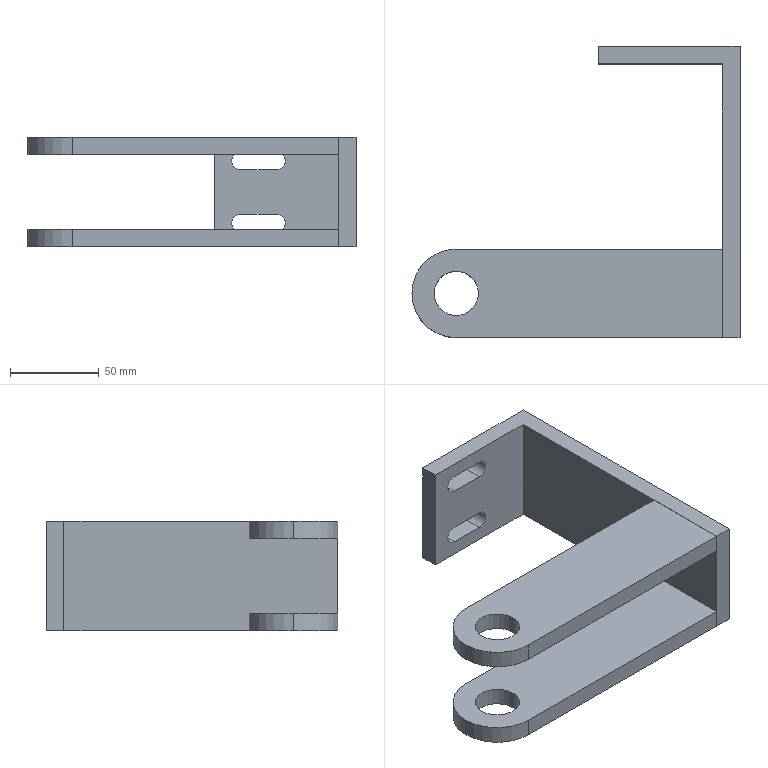Part | SolidWorks | features ICE 3, Extrusion 1, MirrorSolid 1, Split 1 | 3 solids | 34 faces | box 185 x 164.4 x 62 mm | volume 299575 mm3 | plane 22 | cylinder 12 | commonest cylinder face diameters 10 x4 25 x4 50 x4
STEP:
#1=CARTESIAN_POINT('',(-75.,25.,52.));
#2=VERTEX_POINT('',#1);
#3=CARTESIAN_POINT('',(-100.,0.,52.));
#4=VERTEX_POINT('',#3);
#5=CARTESIAN_POINT('',(-75.,0.,52.));
#6=DIRECTION('',(0.,0.,1.));
#7=DIRECTION('',(1.,0.,0.));
#8=AXIS2_PLACEMENT_3D('',#5,#6,#7);
#9=CIRCLE('',#8,25.);
#10=EDGE_CURVE('',#2,#4,#9,.T.);
#11=ORIENTED_EDGE('',*,*,#10,.T.);
#12=CARTESIAN_POINT('',(-100.,0.,62.));
#13=VERTEX_POINT('',#12);
#14=CARTESIAN_POINT('',(-100.,0.,52.));
#15=DIRECTION('',(0.,0.,1.));
#16=VECTOR('',#15,1000.);
#17=LINE('',#14,#16);
#18=EDGE_CURVE('',#4,#13,#17,.T.);
#19=ORIENTED_EDGE('',*,*,#18,.T.);
#20=CARTESIAN_POINT('',(-75.,25.,62.));
#21=VERTEX_POINT('',#20);
#22=CARTESIAN_POINT('',(-75.,0.,62.));
#23=DIRECTION('',(0.,0.,1.));
#24=DIRECTION('',(1.,0.,0.));
#25=AXIS2_PLACEMENT_3D('',#22,#23,#24);
#26=CIRCLE('',#25,25.);
#27=EDGE_CURVE('',#21,#13,#26,.T.);
#28=ORIENTED_EDGE('',*,*,#27,.F.);
#29=CARTESIAN_POINT('',(-75.,25.,52.));
#30=DIRECTION('',(0.,0.,1.));
#31=VECTOR('',#30,1000.);
#32=LINE('',#29,#31);
#33=EDGE_CURVE('',#2,#21,#32,.T.);
#34=ORIENTED_EDGE('',*,*,#33,.F.);
#35=EDGE_LOOP('',(#11,#19,#28,#34));
#36=FACE_OUTER_BOUND('',#35,.T.);
#37=CARTESIAN_POINT('',(-75.,0.,52.));
#38=DIRECTION('',(0.,0.,1.));
#39=DIRECTION('',(-1.,0.,0.));
#40=AXIS2_PLACEMENT_3D('',#37,#38,#39);
#41=CYLINDRICAL_SURFACE('',#40,25.);
#42=ADVANCED_FACE('',(#36),#41,.T.);
#43=CARTESIAN_POINT('',(-62.5,0.,52.));
#44=VERTEX_POINT('',#43);
#45=CARTESIAN_POINT('',(-87.5,0.,52.));
#46=VERTEX_POINT('',#45);
#47=CARTESIAN_POINT('',(-75.,0.,52.));
#48=DIRECTION('',(0.,0.,1.));
#49=DIRECTION('',(1.,0.,0.));
#50=AXIS2_PLACEMENT_3D('',#47,#48,#49);
#51=CIRCLE('',#50,12.5);
#52=EDGE_CURVE('',#44,#46,#51,.T.);
#53=ORIENTED_EDGE('',*,*,#52,.F.);
#54=CARTESIAN_POINT('',(-62.5,0.,62.));
#55=VERTEX_POINT('',#54);
#56=CARTESIAN_POINT('',(-62.5,0.,52.));
#57=DIRECTION('',(0.,0.,1.));
#58=VECTOR('',#57,1000.);
#59=LINE('',#56,#58);
#60=EDGE_CURVE('',#44,#55,#59,.T.);
#61=ORIENTED_EDGE('',*,*,#60,.T.);
#62=CARTESIAN_POINT('',(-87.5,0.,62.));
#63=VERTEX_POINT('',#62);
#64=CARTESIAN_POINT('',(-75.,0.,62.));
#65=DIRECTION('',(0.,0.,1.));
#66=DIRECTION('',(1.,0.,0.));
#67=AXIS2_PLACEMENT_3D('',#64,#65,#66);
#68=CIRCLE('',#67,12.5);
#69=EDGE_CURVE('',#55,#63,#68,.T.);
#70=ORIENTED_EDGE('',*,*,#69,.T.);
#71=CARTESIAN_POINT('',(-87.5,0.,52.));
#72=DIRECTION('',(0.,0.,1.));
#73=VECTOR('',#72,1000.);
#74=LINE('',#71,#73);
#75=EDGE_CURVE('',#46,#63,#74,.T.);
#76=ORIENTED_EDGE('',*,*,#75,.F.);
#77=EDGE_LOOP('',(#53,#61,#70,#76));
#78=FACE_OUTER_BOUND('',#77,.T.);
#79=CARTESIAN_POINT('',(-75.,0.,52.));
#80=DIRECTION('',(0.,0.,1.));
#81=DIRECTION('',(-1.,0.,0.));
#82=AXIS2_PLACEMENT_3D('',#79,#80,#81);
#83=CYLINDRICAL_SURFACE('',#82,12.5);
#84=ADVANCED_FACE('',(#78),#83,.F.);
#85=CARTESIAN_POINT('',(75.,-25.,52.));
#86=VERTEX_POINT('',#85);
#87=CARTESIAN_POINT('',(75.,-25.,62.));
#88=VERTEX_POINT('',#87);
#89=CARTESIAN_POINT('',(75.,-25.,10.));
#90=DIRECTION('',(0.,0.,1.));
#91=VECTOR('',#90,1000.);
#92=LINE('',#89,#91);
#93=EDGE_CURVE('',#86,#88,#92,.T.);
#94=ORIENTED_EDGE('',*,*,#93,.F.);
#95=CARTESIAN_POINT('',(75.,25.,52.));
#96=VERTEX_POINT('',#95);
#97=CARTESIAN_POINT('',(75.,0.,52.));
#98=DIRECTION('',(0.,-1.,0.));
#99=VECTOR('',#98,1000.);
#100=LINE('',#97,#99);
#101=EDGE_CURVE('',#96,#86,#100,.T.);
#102=ORIENTED_EDGE('',*,*,#101,.F.);
#103=CARTESIAN_POINT('',(75.,25.,62.));
#104=VERTEX_POINT('',#103);
#105=CARTESIAN_POINT('',(75.,25.,52.));
#106=DIRECTION('',(0.,0.,1.));
#107=VECTOR('',#106,1000.);
#108=LINE('',#105,#107);
#109=EDGE_CURVE('',#96,#104,#108,.T.);
#110=ORIENTED_EDGE('',*,*,#109,.T.);
#111=CARTESIAN_POINT('',(75.,-25.,62.));
#112=DIRECTION('',(0.,1.,0.));
#113=VECTOR('',#112,1000.);
#114=LINE('',#111,#113);
#115=EDGE_CURVE('',#88,#104,#114,.T.);
#116=ORIENTED_EDGE('',*,*,#115,.F.);
#117=EDGE_LOOP('',(#94,#102,#110,#116));
#118=FACE_OUTER_BOUND('',#117,.T.);
#119=CARTESIAN_POINT('',(75.,129.4,0.));
#120=DIRECTION('',(-1.,0.,0.));
#121=DIRECTION('',(0.,0.,1.));
#122=AXIS2_PLACEMENT_3D('',#119,#120,#121);
#123=PLANE('',#122);
#124=ADVANCED_FACE('',(#118),#123,.F.);
#125=CARTESIAN_POINT('',(-75.,-25.,52.));
#126=VERTEX_POINT('',#125);
#127=CARTESIAN_POINT('',(0.,-25.,52.));
#128=DIRECTION('',(1.,0.,0.));
#129=VECTOR('',#128,1000.);
#130=LINE('',#127,#129);
#131=EDGE_CURVE('',#126,#86,#130,.T.);
#132=ORIENTED_EDGE('',*,*,#131,.F.);
#133=CARTESIAN_POINT('',(-75.,0.,52.));
#134=DIRECTION('',(0.,0.,1.));
#135=DIRECTION('',(1.,0.,0.));
#136=AXIS2_PLACEMENT_3D('',#133,#134,#135);
#137=CIRCLE('',#136,25.);
#138=EDGE_CURVE('',#4,#126,#137,.T.);
#139=ORIENTED_EDGE('',*,*,#138,.F.);
#140=ORIENTED_EDGE('',*,*,#10,.F.);
#141=CARTESIAN_POINT('',(0.,25.,52.));
#142=DIRECTION('',(1.,0.,0.));
#143=VECTOR('',#142,1000.);
#144=LINE('',#141,#143);
#145=EDGE_CURVE('',#2,#96,#144,.T.);
#146=ORIENTED_EDGE('',*,*,#145,.T.);
#147=ORIENTED_EDGE('',*,*,#101,.T.);
#148=EDGE_LOOP('',(#132,#139,#140,#146,#147));
#149=FACE_OUTER_BOUND('',#148,.T.);
#150=CARTESIAN_POINT('',(-75.,0.,52.));
#151=DIRECTION('',(0.,0.,1.));
#152=DIRECTION('',(1.,0.,0.));
#153=AXIS2_PLACEMENT_3D('',#150,#151,#152);
#154=CIRCLE('',#153,12.5);
#155=EDGE_CURVE('',#46,#44,#154,.T.);
#156=ORIENTED_EDGE('',*,*,#155,.T.);
#157=ORIENTED_EDGE('',*,*,#52,.T.);
#158=EDGE_LOOP('',(#156,#157));
#159=FACE_BOUND('',#158,.T.);
#160=CARTESIAN_POINT('',(0.,0.,52.));
#161=DIRECTION('',(0.,0.,-1.));
#162=DIRECTION('',(1.,0.,0.));
#163=AXIS2_PLACEMENT_3D('',#160,#161,#162);
#164=PLANE('',#163);
#165=ADVANCED_FACE('',(#149,#159),#164,.T.);
#166=ORIENTED_EDGE('',*,*,#131,.T.);
#167=ORIENTED_EDGE('',*,*,#93,.T.);
#168=CARTESIAN_POINT('',(-75.,-25.,62.));
#169=VERTEX_POINT('',#168);
#170=CARTESIAN_POINT('',(85.,-25.,62.));
#171=DIRECTION('',(-1.,0.,0.));
#172=VECTOR('',#171,1000.);
#173=LINE('',#170,#172);
#174=EDGE_CURVE('',#88,#169,#173,.T.);
#175=ORIENTED_EDGE('',*,*,#174,.T.);
#176=CARTESIAN_POINT('',(-75.,-25.,52.));
#177=DIRECTION('',(0.,0.,1.));
#178=VECTOR('',#177,1000.);
#179=LINE('',#176,#178);
#180=EDGE_CURVE('',#126,#169,#179,.T.);
#181=ORIENTED_EDGE('',*,*,#180,.F.);
#182=EDGE_LOOP('',(#166,#167,#175,#181));
#183=FACE_OUTER_BOUND('',#182,.T.);
#184=CARTESIAN_POINT('',(0.,-25.,10.));
#185=DIRECTION('',(0.,1.,0.));
#186=DIRECTION('',(-1.,0.,0.));
#187=AXIS2_PLACEMENT_3D('',#184,#185,#186);
#188=PLANE('',#187);
#189=ADVANCED_FACE('',(#183),#188,.F.);
#190=ORIENTED_EDGE('',*,*,#18,.F.);
#191=ORIENTED_EDGE('',*,*,#138,.T.);
#192=ORIENTED_EDGE('',*,*,#180,.T.);
#193=CARTESIAN_POINT('',(-75.,0.,62.));
#194=DIRECTION('',(0.,0.,1.));
#195=DIRECTION('',(1.,0.,0.));
#196=AXIS2_PLACEMENT_3D('',#193,#194,#195);
#197=CIRCLE('',#196,25.);
#198=EDGE_CURVE('',#13,#169,#197,.T.);
#199=ORIENTED_EDGE('',*,*,#198,.F.);
#200=EDGE_LOOP('',(#190,#191,#192,#199));
#201=FACE_OUTER_BOUND('',#200,.T.);
#202=CARTESIAN_POINT('',(-75.,0.,52.));
#203=DIRECTION('',(0.,0.,1.));
#204=DIRECTION('',(-1.,0.,0.));
#205=AXIS2_PLACEMENT_3D('',#202,#203,#204);
#206=CYLINDRICAL_SURFACE('',#205,25.);
#207=ADVANCED_FACE('',(#201),#206,.T.);
#208=CARTESIAN_POINT('',(0.,25.,62.));
#209=DIRECTION('',(1.,0.,0.));
#210=VECTOR('',#209,1000.);
#211=LINE('',#208,#210);
#212=EDGE_CURVE('',#21,#104,#211,.T.);
#213=ORIENTED_EDGE('',*,*,#212,.T.);
#214=ORIENTED_EDGE('',*,*,#109,.F.);
#215=ORIENTED_EDGE('',*,*,#145,.F.);
#216=ORIENTED_EDGE('',*,*,#33,.T.);
#217=EDGE_LOOP('',(#213,#214,#215,#216));
#218=FACE_OUTER_BOUND('',#217,.T.);
#219=CARTESIAN_POINT('',(0.,25.,52.));
#220=DIRECTION('',(0.,1.,0.));
#221=DIRECTION('',(-1.,0.,0.));
#222=AXIS2_PLACEMENT_3D('',#219,#220,#221);
#223=PLANE('',#222);
#224=ADVANCED_FACE('',(#218),#223,.T.);
#225=ORIENTED_EDGE('',*,*,#60,.F.);
#226=ORIENTED_EDGE('',*,*,#155,.F.);
#227=ORIENTED_EDGE('',*,*,#75,.T.);
#228=CARTESIAN_POINT('',(-75.,0.,62.));
#229=DIRECTION('',(0.,0.,1.));
#230=DIRECTION('',(1.,0.,0.));
#231=AXIS2_PLACEMENT_3D('',#228,#229,#230);
#232=CIRCLE('',#231,12.5);
#233=EDGE_CURVE('',#63,#55,#232,.T.);
#234=ORIENTED_EDGE('',*,*,#233,.T.);
#235=EDGE_LOOP('',(#225,#226,#227,#234));
#236=FACE_OUTER_BOUND('',#235,.T.);
#237=CARTESIAN_POINT('',(-75.,0.,52.));
#238=DIRECTION('',(0.,0.,1.));
#239=DIRECTION('',(-1.,0.,0.));
#240=AXIS2_PLACEMENT_3D('',#237,#238,#239);
#241=CYLINDRICAL_SURFACE('',#240,12.5);
#242=ADVANCED_FACE('',(#236),#241,.F.);
#243=ORIENTED_EDGE('',*,*,#233,.F.);
#244=ORIENTED_EDGE('',*,*,#69,.F.);
#245=EDGE_LOOP('',(#243,#244));
#246=FACE_BOUND('',#245,.T.);
#247=ORIENTED_EDGE('',*,*,#174,.F.);
#248=ORIENTED_EDGE('',*,*,#115,.T.);
#249=ORIENTED_EDGE('',*,*,#212,.F.);
#250=ORIENTED_EDGE('',*,*,#27,.T.);
#251=ORIENTED_EDGE('',*,*,#198,.T.);
#252=EDGE_LOOP('',(#247,#248,#249,#250,#251));
#253=FACE_OUTER_BOUND('',#252,.T.);
#254=CARTESIAN_POINT('',(85.,-25.,62.));
#255=DIRECTION('',(0.,0.,-1.));
#256=DIRECTION('',(-1.,0.,0.));
#257=AXIS2_PLACEMENT_3D('',#254,#255,#256);
#258=PLANE('',#257);
#259=ADVANCED_FACE('',(#246,#253),#258,.F.);
#260=CLOSED_SHELL('',(#42,#84,#124,#165,#189,#207,#224,#242,#259));
#261=MANIFOLD_SOLID_BREP('',#260);
#262=CARTESIAN_POINT('',(-87.5,0.,10.));
#263=VERTEX_POINT('',#262);
#264=CARTESIAN_POINT('',(-62.5,0.,10.));
#265=VERTEX_POINT('',#264);
#266=CARTESIAN_POINT('',(-75.,0.,10.));
#267=DIRECTION('',(0.,0.,1.));
#268=DIRECTION('',(1.,0.,0.));
#269=AXIS2_PLACEMENT_3D('',#266,#267,#268);
#270=CIRCLE('',#269,12.5);
#271=EDGE_CURVE('',#263,#265,#270,.T.);
#272=ORIENTED_EDGE('',*,*,#271,.T.);
#273=CARTESIAN_POINT('',(-62.5,0.,0.));
#274=VERTEX_POINT('',#273);
#275=CARTESIAN_POINT('',(-62.5,0.,10.));
#276=DIRECTION('',(0.,0.,-1.));
#277=VECTOR('',#276,1000.);
#278=LINE('',#275,#277);
#279=EDGE_CURVE('',#265,#274,#278,.T.);
#280=ORIENTED_EDGE('',*,*,#279,.T.);
#281=CARTESIAN_POINT('',(-87.5,0.,0.));
#282=VERTEX_POINT('',#281);
#283=CARTESIAN_POINT('',(-75.,0.,0.));
#284=DIRECTION('',(0.,0.,1.));
#285=DIRECTION('',(1.,0.,0.));
#286=AXIS2_PLACEMENT_3D('',#283,#284,#285);
#287=CIRCLE('',#286,12.5);
#288=EDGE_CURVE('',#282,#274,#287,.T.);
#289=ORIENTED_EDGE('',*,*,#288,.F.);
#290=CARTESIAN_POINT('',(-87.5,0.,10.));
#291=DIRECTION('',(0.,0.,-1.));
#292=VECTOR('',#291,1000.);
#293=LINE('',#290,#292);
#294=EDGE_CURVE('',#263,#282,#293,.T.);
#295=ORIENTED_EDGE('',*,*,#294,.F.);
#296=EDGE_LOOP('',(#272,#280,#289,#295));
#297=FACE_OUTER_BOUND('',#296,.T.);
#298=CARTESIAN_POINT('',(-75.,0.,10.));
#299=DIRECTION('',(0.,0.,-1.));
#300=DIRECTION('',(-1.,0.,0.));
#301=AXIS2_PLACEMENT_3D('',#298,#299,#300);
#302=CYLINDRICAL_SURFACE('',#301,12.5);
#303=ADVANCED_FACE('',(#297),#302,.F.);
#304=CARTESIAN_POINT('',(-100.,0.,10.));
#305=VERTEX_POINT('',#304);
#306=CARTESIAN_POINT('',(-75.,-25.,10.));
#307=VERTEX_POINT('',#306);
#308=CARTESIAN_POINT('',(-75.,0.,10.));
#309=DIRECTION('',(0.,0.,1.));
#310=DIRECTION('',(1.,0.,0.));
#311=AXIS2_PLACEMENT_3D('',#308,#309,#310);
#312=CIRCLE('',#311,25.);
#313=EDGE_CURVE('',#305,#307,#312,.T.);
#314=ORIENTED_EDGE('',*,*,#313,.F.);
#315=CARTESIAN_POINT('',(-100.,0.,0.));
#316=VERTEX_POINT('',#315);
#317=CARTESIAN_POINT('',(-100.,0.,10.));
#318=DIRECTION('',(0.,0.,-1.));
#319=VECTOR('',#318,1000.);
#320=LINE('',#317,#319);
#321=EDGE_CURVE('',#305,#316,#320,.T.);
#322=ORIENTED_EDGE('',*,*,#321,.T.);
#323=CARTESIAN_POINT('',(-75.,-25.,0.));
#324=VERTEX_POINT('',#323);
#325=CARTESIAN_POINT('',(-75.,0.,0.));
#326=DIRECTION('',(0.,0.,1.));
#327=DIRECTION('',(1.,0.,0.));
#328=AXIS2_PLACEMENT_3D('',#325,#326,#327);
#329=CIRCLE('',#328,25.);
#330=EDGE_CURVE('',#316,#324,#329,.T.);
#331=ORIENTED_EDGE('',*,*,#330,.T.);
#332=CARTESIAN_POINT('',(-75.,-25.,10.));
#333=DIRECTION('',(0.,0.,-1.));
#334=VECTOR('',#333,1000.);
#335=LINE('',#332,#334);
#336=EDGE_CURVE('',#307,#324,#335,.T.);
#337=ORIENTED_EDGE('',*,*,#336,.F.);
#338=EDGE_LOOP('',(#314,#322,#331,#337));
#339=FACE_OUTER_BOUND('',#338,.T.);
#340=CARTESIAN_POINT('',(-75.,0.,10.));
#341=DIRECTION('',(0.,0.,-1.));
#342=DIRECTION('',(-1.,0.,0.));
#343=AXIS2_PLACEMENT_3D('',#340,#341,#342);
#344=CYLINDRICAL_SURFACE('',#343,25.);
#345=ADVANCED_FACE('',(#339),#344,.T.);
#346=CARTESIAN_POINT('',(75.,25.,0.));
#347=VERTEX_POINT('',#346);
#348=CARTESIAN_POINT('',(75.,-25.,0.));
#349=VERTEX_POINT('',#348);
#350=CARTESIAN_POINT('',(75.,0.,0.));
#351=DIRECTION('',(0.,-1.,0.));
#352=VECTOR('',#351,1000.);
#353=LINE('',#350,#352);
#354=EDGE_CURVE('',#347,#349,#353,.T.);
#355=ORIENTED_EDGE('',*,*,#354,.F.);
#356=CARTESIAN_POINT('',(75.,25.,10.));
#357=VERTEX_POINT('',#356);
#358=CARTESIAN_POINT('',(75.,25.,10.));
#359=DIRECTION('',(0.,0.,-1.));
#360=VECTOR('',#359,1000.);
#361=LINE('',#358,#360);
#362=EDGE_CURVE('',#357,#347,#361,.T.);
#363=ORIENTED_EDGE('',*,*,#362,.F.);
#364=CARTESIAN_POINT('',(75.,-25.,10.));
#365=VERTEX_POINT('',#364);
#366=CARTESIAN_POINT('',(75.,0.,10.));
#367=DIRECTION('',(0.,-1.,0.));
#368=VECTOR('',#367,1000.);
#369=LINE('',#366,#368);
#370=EDGE_CURVE('',#357,#365,#369,.T.);
#371=ORIENTED_EDGE('',*,*,#370,.T.);
#372=CARTESIAN_POINT('',(75.,-25.,10.));
#373=DIRECTION('',(0.,0.,1.));
#374=VECTOR('',#373,1000.);
#375=LINE('',#372,#374);
#376=EDGE_CURVE('',#349,#365,#375,.T.);
#377=ORIENTED_EDGE('',*,*,#376,.F.);
#378=EDGE_LOOP('',(#355,#363,#371,#377));
#379=FACE_OUTER_BOUND('',#378,.T.);
#380=CARTESIAN_POINT('',(75.,129.4,0.));
#381=DIRECTION('',(-1.,0.,0.));
#382=DIRECTION('',(0.,0.,1.));
#383=AXIS2_PLACEMENT_3D('',#380,#381,#382);
#384=PLANE('',#383);
#385=ADVANCED_FACE('',(#379),#384,.F.);
#386=CARTESIAN_POINT('',(-75.,25.,0.));
#387=VERTEX_POINT('',#386);
#388=CARTESIAN_POINT('',(0.,25.,0.));
#389=DIRECTION('',(1.,0.,0.));
#390=VECTOR('',#389,1000.);
#391=LINE('',#388,#390);
#392=EDGE_CURVE('',#387,#347,#391,.T.);
#393=ORIENTED_EDGE('',*,*,#392,.T.);
#394=ORIENTED_EDGE('',*,*,#354,.T.);
#395=CARTESIAN_POINT('',(0.,-25.,0.));
#396=DIRECTION('',(1.,0.,0.));
#397=VECTOR('',#396,1000.);
#398=LINE('',#395,#397);
#399=EDGE_CURVE('',#324,#349,#398,.T.);
#400=ORIENTED_EDGE('',*,*,#399,.F.);
#401=ORIENTED_EDGE('',*,*,#330,.F.);
#402=CARTESIAN_POINT('',(-75.,0.,0.));
#403=DIRECTION('',(0.,0.,1.));
#404=DIRECTION('',(1.,0.,0.));
#405=AXIS2_PLACEMENT_3D('',#402,#403,#404);
#406=CIRCLE('',#405,25.);
#407=EDGE_CURVE('',#387,#316,#406,.T.);
#408=ORIENTED_EDGE('',*,*,#407,.F.);
#409=EDGE_LOOP('',(#393,#394,#400,#401,#408));
#410=FACE_OUTER_BOUND('',#409,.T.);
#411=ORIENTED_EDGE('',*,*,#288,.T.);
#412=CARTESIAN_POINT('',(-75.,0.,0.));
#413=DIRECTION('',(0.,0.,1.));
#414=DIRECTION('',(1.,0.,0.));
#415=AXIS2_PLACEMENT_3D('',#412,#413,#414);
#416=CIRCLE('',#415,12.5);
#417=EDGE_CURVE('',#274,#282,#416,.T.);
#418=ORIENTED_EDGE('',*,*,#417,.T.);
#419=EDGE_LOOP('',(#411,#418));
#420=FACE_BOUND('',#419,.T.);
#421=CARTESIAN_POINT('',(0.,0.,0.));
#422=DIRECTION('',(0.,0.,1.));
#423=DIRECTION('',(1.,0.,0.));
#424=AXIS2_PLACEMENT_3D('',#421,#422,#423);
#425=PLANE('',#424);
#426=ADVANCED_FACE('',(#410,#420),#425,.F.);
#427=CARTESIAN_POINT('',(0.,-25.,10.));
#428=DIRECTION('',(1.,0.,0.));
#429=VECTOR('',#428,1000.);
#430=LINE('',#427,#429);
#431=EDGE_CURVE('',#307,#365,#430,.T.);
#432=ORIENTED_EDGE('',*,*,#431,.T.);
#433=ORIENTED_EDGE('',*,*,#370,.F.);
#434=CARTESIAN_POINT('',(-75.,25.,10.));
#435=VERTEX_POINT('',#434);
#436=CARTESIAN_POINT('',(0.,25.,10.));
#437=DIRECTION('',(1.,0.,0.));
#438=VECTOR('',#437,1000.);
#439=LINE('',#436,#438);
#440=EDGE_CURVE('',#435,#357,#439,.T.);
#441=ORIENTED_EDGE('',*,*,#440,.F.);
#442=CARTESIAN_POINT('',(-75.,0.,10.));
#443=DIRECTION('',(0.,0.,1.));
#444=DIRECTION('',(1.,0.,0.));
#445=AXIS2_PLACEMENT_3D('',#442,#443,#444);
#446=CIRCLE('',#445,25.);
#447=EDGE_CURVE('',#435,#305,#446,.T.);
#448=ORIENTED_EDGE('',*,*,#447,.T.);
#449=ORIENTED_EDGE('',*,*,#313,.T.);
#450=EDGE_LOOP('',(#432,#433,#441,#448,#449));
#451=FACE_OUTER_BOUND('',#450,.T.);
#452=ORIENTED_EDGE('',*,*,#271,.F.);
#453=CARTESIAN_POINT('',(-75.,0.,10.));
#454=DIRECTION('',(0.,0.,1.));
#455=DIRECTION('',(1.,0.,0.));
#456=AXIS2_PLACEMENT_3D('',#453,#454,#455);
#457=CIRCLE('',#456,12.5);
#458=EDGE_CURVE('',#265,#263,#457,.T.);
#459=ORIENTED_EDGE('',*,*,#458,.F.);
#460=EDGE_LOOP('',(#452,#459));
#461=FACE_BOUND('',#460,.T.);
#462=CARTESIAN_POINT('',(0.,0.,10.));
#463=DIRECTION('',(0.,0.,1.));
#464=DIRECTION('',(1.,0.,0.));
#465=AXIS2_PLACEMENT_3D('',#462,#463,#464);
#466=PLANE('',#465);
#467=ADVANCED_FACE('',(#451,#461),#466,.T.);
#468=ORIENTED_EDGE('',*,*,#279,.F.);
#469=ORIENTED_EDGE('',*,*,#458,.T.);
#470=ORIENTED_EDGE('',*,*,#294,.T.);
#471=ORIENTED_EDGE('',*,*,#417,.F.);
#472=EDGE_LOOP('',(#468,#469,#470,#471));
#473=FACE_OUTER_BOUND('',#472,.T.);
#474=CARTESIAN_POINT('',(-75.,0.,10.));
#475=DIRECTION('',(0.,0.,-1.));
#476=DIRECTION('',(-1.,0.,0.));
#477=AXIS2_PLACEMENT_3D('',#474,#475,#476);
#478=CYLINDRICAL_SURFACE('',#477,12.5);
#479=ADVANCED_FACE('',(#473),#478,.F.);
#480=ORIENTED_EDGE('',*,*,#321,.F.);
#481=ORIENTED_EDGE('',*,*,#447,.F.);
#482=CARTESIAN_POINT('',(-75.,25.,10.));
#483=DIRECTION('',(0.,0.,-1.));
#484=VECTOR('',#483,1000.);
#485=LINE('',#482,#484);
#486=EDGE_CURVE('',#435,#387,#485,.T.);
#487=ORIENTED_EDGE('',*,*,#486,.T.);
#488=ORIENTED_EDGE('',*,*,#407,.T.);
#489=EDGE_LOOP('',(#480,#481,#487,#488));
#490=FACE_OUTER_BOUND('',#489,.T.);
#491=CARTESIAN_POINT('',(-75.,0.,10.));
#492=DIRECTION('',(0.,0.,-1.));
#493=DIRECTION('',(-1.,0.,0.));
#494=AXIS2_PLACEMENT_3D('',#491,#492,#493);
#495=CYLINDRICAL_SURFACE('',#494,25.);
#496=ADVANCED_FACE('',(#490),#495,.T.);
#497=ORIENTED_EDGE('',*,*,#392,.F.);
#498=ORIENTED_EDGE('',*,*,#486,.F.);
#499=ORIENTED_EDGE('',*,*,#440,.T.);
#500=ORIENTED_EDGE('',*,*,#362,.T.);
#501=EDGE_LOOP('',(#497,#498,#499,#500));
#502=FACE_OUTER_BOUND('',#501,.T.);
#503=CARTESIAN_POINT('',(0.,25.,10.));
#504=DIRECTION('',(0.,1.,0.));
#505=DIRECTION('',(-1.,0.,0.));
#506=AXIS2_PLACEMENT_3D('',#503,#504,#505);
#507=PLANE('',#506);
#508=ADVANCED_FACE('',(#502),#507,.T.);
#509=ORIENTED_EDGE('',*,*,#399,.T.);
#510=ORIENTED_EDGE('',*,*,#376,.T.);
#511=ORIENTED_EDGE('',*,*,#431,.F.);
#512=ORIENTED_EDGE('',*,*,#336,.T.);
#513=EDGE_LOOP('',(#509,#510,#511,#512));
#514=FACE_OUTER_BOUND('',#513,.T.);
#515=CARTESIAN_POINT('',(0.,-25.,10.));
#516=DIRECTION('',(0.,1.,0.));
#517=DIRECTION('',(-1.,0.,0.));
#518=AXIS2_PLACEMENT_3D('',#515,#516,#517);
#519=PLANE('',#518);
#520=ADVANCED_FACE('',(#514),#519,.F.);
#521=CLOSED_SHELL('',(#303,#345,#385,#426,#467,#479,#496,#508,#520));
#522=MANIFOLD_SOLID_BREP('',#521);
#523=CARTESIAN_POINT('',(40.,129.4,43.5));
#524=VERTEX_POINT('',#523);
#525=CARTESIAN_POINT('',(20.,129.4,43.5));
#526=VERTEX_POINT('',#525);
#527=CARTESIAN_POINT('',(20.,129.4,43.5));
#528=DIRECTION('',(-1.,0.,0.));
#529=VECTOR('',#528,1000.);
#530=LINE('',#527,#529);
#531=EDGE_CURVE('',#524,#526,#530,.T.);
#532=ORIENTED_EDGE('',*,*,#531,.T.);
#533=CARTESIAN_POINT('',(20.,129.4,53.5));
#534=VERTEX_POINT('',#533);
#535=CARTESIAN_POINT('',(20.,129.4,48.5));
#536=DIRECTION('',(0.,1.,0.));
#537=DIRECTION('',(0.,0.,1.));
#538=AXIS2_PLACEMENT_3D('',#535,#536,#537);
#539=CIRCLE('',#538,5.);
#540=EDGE_CURVE('',#526,#534,#539,.T.);
#541=ORIENTED_EDGE('',*,*,#540,.T.);
#542=CARTESIAN_POINT('',(40.,129.4,53.5));
#543=VERTEX_POINT('',#542);
#544=CARTESIAN_POINT('',(20.,129.4,53.5));
#545=DIRECTION('',(1.,0.,0.));
#546=VECTOR('',#545,1000.);
#547=LINE('',#544,#546);
#548=EDGE_CURVE('',#534,#543,#547,.T.);
#549=ORIENTED_EDGE('',*,*,#548,.T.);
#550=CARTESIAN_POINT('',(40.,129.4,48.5));
#551=DIRECTION('',(0.,1.,0.));
#552=DIRECTION('',(0.,0.,1.));
#553=AXIS2_PLACEMENT_3D('',#550,#551,#552);
#554=CIRCLE('',#553,5.);
#555=EDGE_CURVE('',#543,#524,#554,.T.);
#556=ORIENTED_EDGE('',*,*,#555,.T.);
#557=EDGE_LOOP('',(#532,#541,#549,#556));
#558=FACE_BOUND('',#557,.T.);
#559=CARTESIAN_POINT('',(40.,129.4,8.5));
#560=VERTEX_POINT('',#559);
#561=CARTESIAN_POINT('',(20.,129.4,8.5));
#562=VERTEX_POINT('',#561);
#563=CARTESIAN_POINT('',(20.,129.4,8.5));
#564=DIRECTION('',(-1.,0.,0.));
#565=VECTOR('',#564,1000.);
#566=LINE('',#563,#565);
#567=EDGE_CURVE('',#560,#562,#566,.T.);
#568=ORIENTED_EDGE('',*,*,#567,.T.);
#569=CARTESIAN_POINT('',(20.,129.4,18.5));
#570=VERTEX_POINT('',#569);
#571=CARTESIAN_POINT('',(20.,129.4,13.5));
#572=DIRECTION('',(0.,1.,0.));
#573=DIRECTION('',(0.,0.,1.));
#574=AXIS2_PLACEMENT_3D('',#571,#572,#573);
#575=CIRCLE('',#574,5.);
#576=EDGE_CURVE('',#562,#570,#575,.T.);
#577=ORIENTED_EDGE('',*,*,#576,.T.);
#578=CARTESIAN_POINT('',(40.,129.4,18.5));
#579=VERTEX_POINT('',#578);
#580=CARTESIAN_POINT('',(20.,129.4,18.5));
#581=DIRECTION('',(1.,0.,0.));
#582=VECTOR('',#581,1000.);
#583=LINE('',#580,#582);
#584=EDGE_CURVE('',#570,#579,#583,.T.);
#585=ORIENTED_EDGE('',*,*,#584,.T.);
#586=CARTESIAN_POINT('',(40.,129.4,13.5));
#587=DIRECTION('',(0.,1.,0.));
#588=DIRECTION('',(0.,0.,1.));
#589=AXIS2_PLACEMENT_3D('',#586,#587,#588);
#590=CIRCLE('',#589,5.);
#591=EDGE_CURVE('',#579,#560,#590,.T.);
#592=ORIENTED_EDGE('',*,*,#591,.T.);
#593=EDGE_LOOP('',(#568,#577,#585,#592));
#594=FACE_BOUND('',#593,.T.);
#595=CARTESIAN_POINT('',(75.,129.4,0.));
#596=VERTEX_POINT('',#595);
#597=CARTESIAN_POINT('',(5.,129.4,0.));
#598=VERTEX_POINT('',#597);
#599=CARTESIAN_POINT('',(5.,129.4,0.));
#600=DIRECTION('',(-1.,0.,0.));
#601=VECTOR('',#600,1000.);
#602=LINE('',#599,#601);
#603=EDGE_CURVE('',#596,#598,#602,.T.);
#604=ORIENTED_EDGE('',*,*,#603,.F.);
#605=CARTESIAN_POINT('',(75.,129.4,62.));
#606=VERTEX_POINT('',#605);
#607=CARTESIAN_POINT('',(75.,129.4,0.));
#608=DIRECTION('',(0.,0.,1.));
#609=VECTOR('',#608,1000.);
#610=LINE('',#607,#609);
#611=EDGE_CURVE('',#596,#606,#610,.T.);
#612=ORIENTED_EDGE('',*,*,#611,.T.);
#613=CARTESIAN_POINT('',(5.,129.4,62.));
#614=VERTEX_POINT('',#613);
#615=CARTESIAN_POINT('',(5.,129.4,62.));
#616=DIRECTION('',(1.,0.,0.));
#617=VECTOR('',#616,1000.);
#618=LINE('',#615,#617);
#619=EDGE_CURVE('',#614,#606,#618,.T.);
#620=ORIENTED_EDGE('',*,*,#619,.F.);
#621=CARTESIAN_POINT('',(5.,129.4,0.));
#622=DIRECTION('',(0.,0.,1.));
#623=VECTOR('',#622,1000.);
#624=LINE('',#621,#623);
#625=EDGE_CURVE('',#598,#614,#624,.T.);
#626=ORIENTED_EDGE('',*,*,#625,.F.);
#627=EDGE_LOOP('',(#604,#612,#620,#626));
#628=FACE_OUTER_BOUND('',#627,.T.);
#629=CARTESIAN_POINT('',(0.,129.4,0.));
#630=DIRECTION('',(0.,1.,0.));
#631=DIRECTION('',(0.,0.,1.));
#632=AXIS2_PLACEMENT_3D('',#629,#630,#631);
#633=PLANE('',#632);
#634=ADVANCED_FACE('',(#558,#594,#628),#633,.F.);
#635=CARTESIAN_POINT('',(40.,139.4,43.5));
#636=VERTEX_POINT('',#635);
#637=CARTESIAN_POINT('',(20.,139.4,43.5));
#638=VERTEX_POINT('',#637);
#639=CARTESIAN_POINT('',(20.,139.4,43.5));
#640=DIRECTION('',(-1.,0.,0.));
#641=VECTOR('',#640,1000.);
#642=LINE('',#639,#641);
#643=EDGE_CURVE('',#636,#638,#642,.T.);
#644=ORIENTED_EDGE('',*,*,#643,.T.);
#645=CARTESIAN_POINT('',(20.,129.4,43.5));
#646=DIRECTION('',(0.,1.,0.));
#647=VECTOR('',#646,1000.);
#648=LINE('',#645,#647);
#649=EDGE_CURVE('',#526,#638,#648,.T.);
#650=ORIENTED_EDGE('',*,*,#649,.F.);
#651=ORIENTED_EDGE('',*,*,#531,.F.);
#652=CARTESIAN_POINT('',(40.,129.4,43.5));
#653=DIRECTION('',(0.,1.,0.));
#654=VECTOR('',#653,1000.);
#655=LINE('',#652,#654);
#656=EDGE_CURVE('',#524,#636,#655,.T.);
#657=ORIENTED_EDGE('',*,*,#656,.T.);
#658=EDGE_LOOP('',(#644,#650,#651,#657));
#659=FACE_OUTER_BOUND('',#658,.T.);
#660=CARTESIAN_POINT('',(20.,129.4,43.5));
#661=DIRECTION('',(0.,0.,-1.));
#662=DIRECTION('',(-1.,0.,0.));
#663=AXIS2_PLACEMENT_3D('',#660,#661,#662);
#664=PLANE('',#663);
#665=ADVANCED_FACE('',(#659),#664,.F.);
#666=CARTESIAN_POINT('',(20.,139.4,53.5));
#667=VERTEX_POINT('',#666);
#668=CARTESIAN_POINT('',(20.,139.4,48.5));
#669=DIRECTION('',(0.,1.,0.));
#670=DIRECTION('',(0.,0.,1.));
#671=AXIS2_PLACEMENT_3D('',#668,#669,#670);
#672=CIRCLE('',#671,5.);
#673=EDGE_CURVE('',#638,#667,#672,.T.);
#674=ORIENTED_EDGE('',*,*,#673,.T.);
#675=CARTESIAN_POINT('',(20.,129.4,53.5));
#676=DIRECTION('',(0.,1.,0.));
#677=VECTOR('',#676,1000.);
#678=LINE('',#675,#677);
#679=EDGE_CURVE('',#534,#667,#678,.T.);
#680=ORIENTED_EDGE('',*,*,#679,.F.);
#681=ORIENTED_EDGE('',*,*,#540,.F.);
#682=ORIENTED_EDGE('',*,*,#649,.T.);
#683=EDGE_LOOP('',(#674,#680,#681,#682));
#684=FACE_OUTER_BOUND('',#683,.T.);
#685=CARTESIAN_POINT('',(20.,129.4,48.5));
#686=DIRECTION('',(0.,1.,0.));
#687=DIRECTION('',(0.,0.,1.));
#688=AXIS2_PLACEMENT_3D('',#685,#686,#687);
#689=CYLINDRICAL_SURFACE('',#688,5.);
#690=ADVANCED_FACE('',(#684),#689,.F.);
#691=CARTESIAN_POINT('',(40.,139.4,53.5));
#692=VERTEX_POINT('',#691);
#693=CARTESIAN_POINT('',(20.,139.4,53.5));
#694=DIRECTION('',(1.,0.,0.));
#695=VECTOR('',#694,1000.);
#696=LINE('',#693,#695);
#697=EDGE_CURVE('',#667,#692,#696,.T.);
#698=ORIENTED_EDGE('',*,*,#697,.T.);
#699=CARTESIAN_POINT('',(40.,129.4,53.5));
#700=DIRECTION('',(0.,1.,0.));
#701=VECTOR('',#700,1000.);
#702=LINE('',#699,#701);
#703=EDGE_CURVE('',#543,#692,#702,.T.);
#704=ORIENTED_EDGE('',*,*,#703,.F.);
#705=ORIENTED_EDGE('',*,*,#548,.F.);
#706=ORIENTED_EDGE('',*,*,#679,.T.);
#707=EDGE_LOOP('',(#698,#704,#705,#706));
#708=FACE_OUTER_BOUND('',#707,.T.);
#709=CARTESIAN_POINT('',(20.,129.4,53.5));
#710=DIRECTION('',(0.,0.,1.));
#711=DIRECTION('',(1.,0.,0.));
#712=AXIS2_PLACEMENT_3D('',#709,#710,#711);
#713=PLANE('',#712);
#714=ADVANCED_FACE('',(#708),#713,.F.);
#715=CARTESIAN_POINT('',(40.,139.4,48.5));
#716=DIRECTION('',(0.,1.,0.));
#717=DIRECTION('',(0.,0.,1.));
#718=AXIS2_PLACEMENT_3D('',#715,#716,#717);
#719=CIRCLE('',#718,5.);
#720=EDGE_CURVE('',#692,#636,#719,.T.);
#721=ORIENTED_EDGE('',*,*,#720,.T.);
#722=ORIENTED_EDGE('',*,*,#656,.F.);
#723=ORIENTED_EDGE('',*,*,#555,.F.);
#724=ORIENTED_EDGE('',*,*,#703,.T.);
#725=EDGE_LOOP('',(#721,#722,#723,#724));
#726=FACE_OUTER_BOUND('',#725,.T.);
#727=CARTESIAN_POINT('',(40.,129.4,48.5));
#728=DIRECTION('',(0.,1.,0.));
#729=DIRECTION('',(0.,0.,1.));
#730=AXIS2_PLACEMENT_3D('',#727,#728,#729);
#731=CYLINDRICAL_SURFACE('',#730,5.);
#732=ADVANCED_FACE('',(#726),#731,.F.);
#733=CARTESIAN_POINT('',(40.,139.4,8.5));
#734=VERTEX_POINT('',#733);
#735=CARTESIAN_POINT('',(20.,139.4,8.5));
#736=VERTEX_POINT('',#735);
#737=CARTESIAN_POINT('',(20.,139.4,8.5));
#738=DIRECTION('',(-1.,0.,0.));
#739=VECTOR('',#738,1000.);
#740=LINE('',#737,#739);
#741=EDGE_CURVE('',#734,#736,#740,.T.);
#742=ORIENTED_EDGE('',*,*,#741,.T.);
#743=CARTESIAN_POINT('',(20.,129.4,8.5));
#744=DIRECTION('',(0.,1.,0.));
#745=VECTOR('',#744,1000.);
#746=LINE('',#743,#745);
#747=EDGE_CURVE('',#562,#736,#746,.T.);
#748=ORIENTED_EDGE('',*,*,#747,.F.);
#749=ORIENTED_EDGE('',*,*,#567,.F.);
#750=CARTESIAN_POINT('',(40.,129.4,8.5));
#751=DIRECTION('',(0.,1.,0.));
#752=VECTOR('',#751,1000.);
#753=LINE('',#750,#752);
#754=EDGE_CURVE('',#560,#734,#753,.T.);
#755=ORIENTED_EDGE('',*,*,#754,.T.);
#756=EDGE_LOOP('',(#742,#748,#749,#755));
#757=FACE_OUTER_BOUND('',#756,.T.);
#758=CARTESIAN_POINT('',(20.,129.4,8.5));
#759=DIRECTION('',(0.,0.,-1.));
#760=DIRECTION('',(-1.,0.,0.));
#761=AXIS2_PLACEMENT_3D('',#758,#759,#760);
#762=PLANE('',#761);
#763=ADVANCED_FACE('',(#757),#762,.F.);
#764=CARTESIAN_POINT('',(20.,139.4,18.5));
#765=VERTEX_POINT('',#764);
#766=CARTESIAN_POINT('',(20.,139.4,13.5));
#767=DIRECTION('',(0.,1.,0.));
#768=DIRECTION('',(0.,0.,1.));
#769=AXIS2_PLACEMENT_3D('',#766,#767,#768);
#770=CIRCLE('',#769,5.);
#771=EDGE_CURVE('',#736,#765,#770,.T.);
#772=ORIENTED_EDGE('',*,*,#771,.T.);
#773=CARTESIAN_POINT('',(20.,129.4,18.5));
#774=DIRECTION('',(0.,1.,0.));
#775=VECTOR('',#774,1000.);
#776=LINE('',#773,#775);
#777=EDGE_CURVE('',#570,#765,#776,.T.);
#778=ORIENTED_EDGE('',*,*,#777,.F.);
#779=ORIENTED_EDGE('',*,*,#576,.F.);
#780=ORIENTED_EDGE('',*,*,#747,.T.);
#781=EDGE_LOOP('',(#772,#778,#779,#780));
#782=FACE_OUTER_BOUND('',#781,.T.);
#783=CARTESIAN_POINT('',(20.,129.4,13.5));
#784=DIRECTION('',(0.,1.,0.));
#785=DIRECTION('',(0.,0.,1.));
#786=AXIS2_PLACEMENT_3D('',#783,#784,#785);
#787=CYLINDRICAL_SURFACE('',#786,5.);
#788=ADVANCED_FACE('',(#782),#787,.F.);
#789=CARTESIAN_POINT('',(40.,139.4,18.5));
#790=VERTEX_POINT('',#789);
#791=CARTESIAN_POINT('',(20.,139.4,18.5));
#792=DIRECTION('',(1.,0.,0.));
#793=VECTOR('',#792,1000.);
#794=LINE('',#791,#793);
#795=EDGE_CURVE('',#765,#790,#794,.T.);
#796=ORIENTED_EDGE('',*,*,#795,.T.);
#797=CARTESIAN_POINT('',(40.,129.4,18.5));
#798=DIRECTION('',(0.,1.,0.));
#799=VECTOR('',#798,1000.);
#800=LINE('',#797,#799);
#801=EDGE_CURVE('',#579,#790,#800,.T.);
#802=ORIENTED_EDGE('',*,*,#801,.F.);
#803=ORIENTED_EDGE('',*,*,#584,.F.);
#804=ORIENTED_EDGE('',*,*,#777,.T.);
#805=EDGE_LOOP('',(#796,#802,#803,#804));
#806=FACE_OUTER_BOUND('',#805,.T.);
#807=CARTESIAN_POINT('',(20.,129.4,18.5));
#808=DIRECTION('',(0.,0.,1.));
#809=DIRECTION('',(1.,0.,0.));
#810=AXIS2_PLACEMENT_3D('',#807,#808,#809);
#811=PLANE('',#810);
#812=ADVANCED_FACE('',(#806),#811,.F.);
#813=CARTESIAN_POINT('',(40.,139.4,13.5));
#814=DIRECTION('',(0.,1.,0.));
#815=DIRECTION('',(0.,0.,1.));
#816=AXIS2_PLACEMENT_3D('',#813,#814,#815);
#817=CIRCLE('',#816,5.);
#818=EDGE_CURVE('',#790,#734,#817,.T.);
#819=ORIENTED_EDGE('',*,*,#818,.T.);
#820=ORIENTED_EDGE('',*,*,#754,.F.);
#821=ORIENTED_EDGE('',*,*,#591,.F.);
#822=ORIENTED_EDGE('',*,*,#801,.T.);
#823=EDGE_LOOP('',(#819,#820,#821,#822));
#824=FACE_OUTER_BOUND('',#823,.T.);
#825=CARTESIAN_POINT('',(40.,129.4,13.5));
#826=DIRECTION('',(0.,1.,0.));
#827=DIRECTION('',(0.,0.,1.));
#828=AXIS2_PLACEMENT_3D('',#825,#826,#827);
#829=CYLINDRICAL_SURFACE('',#828,5.);
#830=ADVANCED_FACE('',(#824),#829,.F.);
#831=CARTESIAN_POINT('',(85.,139.4,0.));
#832=VERTEX_POINT('',#831);
#833=CARTESIAN_POINT('',(5.,139.4,0.));
#834=VERTEX_POINT('',#833);
#835=CARTESIAN_POINT('',(85.,139.4,0.));
#836=DIRECTION('',(-1.,0.,0.));
#837=VECTOR('',#836,1000.);
#838=LINE('',#835,#837);
#839=EDGE_CURVE('',#832,#834,#838,.T.);
#840=ORIENTED_EDGE('',*,*,#839,.F.);
#841=CARTESIAN_POINT('',(85.,-25.,0.));
#842=VERTEX_POINT('',#841);
#843=CARTESIAN_POINT('',(85.,-25.,0.));
#844=DIRECTION('',(0.,1.,0.));
#845=VECTOR('',#844,1000.);
#846=LINE('',#843,#845);
#847=EDGE_CURVE('',#842,#832,#846,.T.);
#848=ORIENTED_EDGE('',*,*,#847,.F.);
#849=CARTESIAN_POINT('',(75.,-25.,0.));
#850=VERTEX_POINT('',#849);
#851=CARTESIAN_POINT('',(0.,-25.,0.));
#852=DIRECTION('',(1.,0.,0.));
#853=VECTOR('',#852,1000.);
#854=LINE('',#851,#853);
#855=EDGE_CURVE('',#850,#842,#854,.T.);
#856=ORIENTED_EDGE('',*,*,#855,.F.);
#857=CARTESIAN_POINT('',(75.,0.,0.));
#858=DIRECTION('',(0.,-1.,0.));
#859=VECTOR('',#858,1000.);
#860=LINE('',#857,#859);
#861=EDGE_CURVE('',#596,#850,#860,.T.);
#862=ORIENTED_EDGE('',*,*,#861,.F.);
#863=ORIENTED_EDGE('',*,*,#603,.T.);
#864=CARTESIAN_POINT('',(5.,129.4,0.));
#865=DIRECTION('',(0.,1.,0.));
#866=VECTOR('',#865,1000.);
#867=LINE('',#864,#866);
#868=EDGE_CURVE('',#598,#834,#867,.T.);
#869=ORIENTED_EDGE('',*,*,#868,.T.);
#870=EDGE_LOOP('',(#840,#848,#856,#862,#863,#869));
#871=FACE_OUTER_BOUND('',#870,.T.);
#872=CARTESIAN_POINT('',(0.,0.,0.));
#873=DIRECTION('',(0.,0.,1.));
#874=DIRECTION('',(1.,0.,0.));
#875=AXIS2_PLACEMENT_3D('',#872,#873,#874);
#876=PLANE('',#875);
#877=ADVANCED_FACE('',(#871),#876,.F.);
#878=CARTESIAN_POINT('',(85.,139.4,62.));
#879=VERTEX_POINT('',#878);
#880=CARTESIAN_POINT('',(85.,-25.,62.));
#881=VERTEX_POINT('',#880);
#882=CARTESIAN_POINT('',(85.,-25.,62.));
#883=DIRECTION('',(0.,-1.,0.));
#884=VECTOR('',#883,1000.);
#885=LINE('',#882,#884);
#886=EDGE_CURVE('',#879,#881,#885,.T.);
#887=ORIENTED_EDGE('',*,*,#886,.F.);
#888=CARTESIAN_POINT('',(5.,139.4,62.));
#889=VERTEX_POINT('',#888);
#890=CARTESIAN_POINT('',(85.,139.4,62.));
#891=DIRECTION('',(-1.,0.,0.));
#892=VECTOR('',#891,1000.);
#893=LINE('',#890,#892);
#894=EDGE_CURVE('',#879,#889,#893,.T.);
#895=ORIENTED_EDGE('',*,*,#894,.T.);
#896=CARTESIAN_POINT('',(5.,129.4,62.));
#897=DIRECTION('',(0.,1.,0.));
#898=VECTOR('',#897,1000.);
#899=LINE('',#896,#898);
#900=EDGE_CURVE('',#614,#889,#899,.T.);
#901=ORIENTED_EDGE('',*,*,#900,.F.);
#902=ORIENTED_EDGE('',*,*,#619,.T.);
#903=CARTESIAN_POINT('',(75.,-25.,62.));
#904=VERTEX_POINT('',#903);
#905=CARTESIAN_POINT('',(75.,-25.,62.));
#906=DIRECTION('',(0.,1.,0.));
#907=VECTOR('',#906,1000.);
#908=LINE('',#905,#907);
#909=EDGE_CURVE('',#904,#606,#908,.T.);
#910=ORIENTED_EDGE('',*,*,#909,.F.);
#911=CARTESIAN_POINT('',(85.,-25.,62.));
#912=DIRECTION('',(-1.,0.,0.));
#913=VECTOR('',#912,1000.);
#914=LINE('',#911,#913);
#915=EDGE_CURVE('',#881,#904,#914,.T.);
#916=ORIENTED_EDGE('',*,*,#915,.F.);
#917=EDGE_LOOP('',(#887,#895,#901,#902,#910,#916));
#918=FACE_OUTER_BOUND('',#917,.T.);
#919=CARTESIAN_POINT('',(85.,-25.,62.));
#920=DIRECTION('',(0.,0.,-1.));
#921=DIRECTION('',(-1.,0.,0.));
#922=AXIS2_PLACEMENT_3D('',#919,#920,#921);
#923=PLANE('',#922);
#924=ADVANCED_FACE('',(#918),#923,.F.);
#925=CARTESIAN_POINT('',(5.,139.4,0.));
#926=DIRECTION('',(0.,0.,1.));
#927=VECTOR('',#926,1000.);
#928=LINE('',#925,#927);
#929=EDGE_CURVE('',#834,#889,#928,.T.);
#930=ORIENTED_EDGE('',*,*,#929,.F.);
#931=ORIENTED_EDGE('',*,*,#868,.F.);
#932=ORIENTED_EDGE('',*,*,#625,.T.);
#933=ORIENTED_EDGE('',*,*,#900,.T.);
#934=EDGE_LOOP('',(#930,#931,#932,#933));
#935=FACE_OUTER_BOUND('',#934,.T.);
#936=CARTESIAN_POINT('',(5.,129.4,0.));
#937=DIRECTION('',(-1.,0.,0.));
#938=DIRECTION('',(0.,0.,1.));
#939=AXIS2_PLACEMENT_3D('',#936,#937,#938);
#940=PLANE('',#939);
#941=ADVANCED_FACE('',(#935),#940,.T.);
#942=ORIENTED_EDGE('',*,*,#894,.F.);
#943=CARTESIAN_POINT('',(85.,139.4,62.));
#944=DIRECTION('',(0.,0.,-1.));
#945=VECTOR('',#944,1000.);
#946=LINE('',#943,#945);
#947=EDGE_CURVE('',#879,#832,#946,.T.);
#948=ORIENTED_EDGE('',*,*,#947,.T.);
#949=ORIENTED_EDGE('',*,*,#839,.T.);
#950=ORIENTED_EDGE('',*,*,#929,.T.);
#951=EDGE_LOOP('',(#942,#948,#949,#950));
#952=FACE_OUTER_BOUND('',#951,.T.);
#953=ORIENTED_EDGE('',*,*,#771,.F.);
#954=ORIENTED_EDGE('',*,*,#741,.F.);
#955=ORIENTED_EDGE('',*,*,#818,.F.);
#956=ORIENTED_EDGE('',*,*,#795,.F.);
#957=EDGE_LOOP('',(#953,#954,#955,#956));
#958=FACE_BOUND('',#957,.T.);
#959=ORIENTED_EDGE('',*,*,#673,.F.);
#960=ORIENTED_EDGE('',*,*,#643,.F.);
#961=ORIENTED_EDGE('',*,*,#720,.F.);
#962=ORIENTED_EDGE('',*,*,#697,.F.);
#963=EDGE_LOOP('',(#959,#960,#961,#962));
#964=FACE_BOUND('',#963,.T.);
#965=CARTESIAN_POINT('',(85.,139.4,0.));
#966=DIRECTION('',(0.,-1.,0.));
#967=DIRECTION('',(0.,0.,-1.));
#968=AXIS2_PLACEMENT_3D('',#965,#966,#967);
#969=PLANE('',#968);
#970=ADVANCED_FACE('',(#952,#958,#964),#969,.F.);
#971=ORIENTED_EDGE('',*,*,#847,.T.);
#972=ORIENTED_EDGE('',*,*,#947,.F.);
#973=ORIENTED_EDGE('',*,*,#886,.T.);
#974=CARTESIAN_POINT('',(85.,-25.,0.));
#975=DIRECTION('',(0.,0.,-1.));
#976=VECTOR('',#975,1000.);
#977=LINE('',#974,#976);
#978=EDGE_CURVE('',#881,#842,#977,.T.);
#979=ORIENTED_EDGE('',*,*,#978,.T.);
#980=EDGE_LOOP('',(#971,#972,#973,#979));
#981=FACE_OUTER_BOUND('',#980,.T.);
#982=CARTESIAN_POINT('',(85.,0.,0.));
#983=DIRECTION('',(1.,0.,0.));
#984=DIRECTION('',(0.,0.,-1.));
#985=AXIS2_PLACEMENT_3D('',#982,#983,#984);
#986=PLANE('',#985);
#987=ADVANCED_FACE('',(#981),#986,.T.);
#988=CARTESIAN_POINT('',(75.,-25.,10.));
#989=DIRECTION('',(0.,0.,1.));
#990=VECTOR('',#989,1000.);
#991=LINE('',#988,#990);
#992=EDGE_CURVE('',#850,#904,#991,.T.);
#993=ORIENTED_EDGE('',*,*,#992,.F.);
#994=ORIENTED_EDGE('',*,*,#855,.T.);
#995=ORIENTED_EDGE('',*,*,#978,.F.);
#996=ORIENTED_EDGE('',*,*,#915,.T.);
#997=EDGE_LOOP('',(#993,#994,#995,#996));
#998=FACE_OUTER_BOUND('',#997,.T.);
#999=CARTESIAN_POINT('',(0.,-25.,10.));
#1000=DIRECTION('',(0.,1.,0.));
#1001=DIRECTION('',(-1.,0.,0.));
#1002=AXIS2_PLACEMENT_3D('',#999,#1000,#1001);
#1003=PLANE('',#1002);
#1004=ADVANCED_FACE('',(#998),#1003,.F.);
#1005=ORIENTED_EDGE('',*,*,#992,.T.);
#1006=ORIENTED_EDGE('',*,*,#909,.T.);
#1007=ORIENTED_EDGE('',*,*,#611,.F.);
#1008=ORIENTED_EDGE('',*,*,#861,.T.);
#1009=EDGE_LOOP('',(#1005,#1006,#1007,#1008));
#1010=FACE_OUTER_BOUND('',#1009,.T.);
#1011=CARTESIAN_POINT('',(75.,129.4,0.));
#1012=DIRECTION('',(-1.,0.,0.));
#1013=DIRECTION('',(0.,0.,1.));
#1014=AXIS2_PLACEMENT_3D('',#1011,#1012,#1013);
#1015=PLANE('',#1014);
#1016=ADVANCED_FACE('',(#1010),#1015,.T.);
#1017=CLOSED_SHELL('',(#634,#665,#690,#714,#732,#763,#788,#812,#830,#877,#924,#941,#970,#987,#1004,#1016));
#1018=MANIFOLD_SOLID_BREP('',#1017);
#1019=CARTESIAN_POINT('',(0.,0.,0.));
#1020=DIRECTION('',(0.,0.,1.));
#1021=DIRECTION('',(1.,0.,0.));
#1022=AXIS2_PLACEMENT_3D('',#1019,#1020,#1021);
#1023=(LENGTH_UNIT()NAMED_UNIT(*)SI_UNIT(.MILLI.,.METRE.));
#1024=UNCERTAINTY_MEASURE_WITH_UNIT(LENGTH_MEASURE(0.00001),#1023,'','');
#1025=(NAMED_UNIT(*)PLANE_ANGLE_UNIT()SI_UNIT($,.RADIAN.));
#1026=(NAMED_UNIT(*)SI_UNIT($,.STERADIAN.)SOLID_ANGLE_UNIT());
#1027=(GEOMETRIC_REPRESENTATION_CONTEXT(3)GLOBAL_UNCERTAINTY_ASSIGNED_CONTEXT((#1024))GLOBAL_UNIT_ASSIGNED_CONTEXT((#1023,#1025,#1026))REPRESENTATION_CONTEXT('',''));
#1028=ADVANCED_BREP_SHAPE_REPRESENTATION('',(#261,#522,#1018,#1022),#1027);